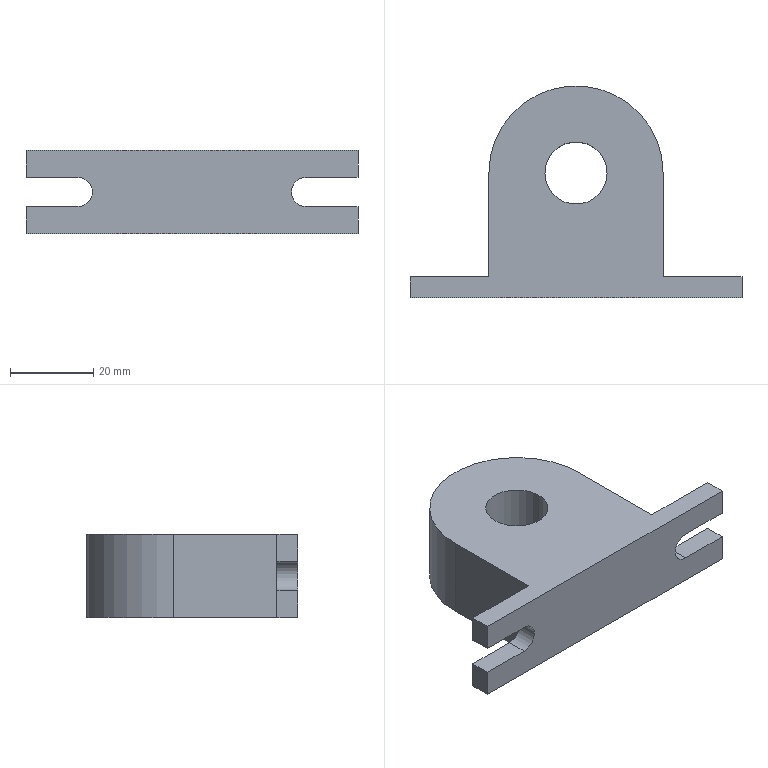Part | SolidWorks | features Extrusion 1, ICE 1 | 1 solid | 21 faces | box 80 x 51 x 20 mm | volume 38253 mm3 | plane 15 | cylinder 6 | commonest cylinder face diameters 7 x3 15 x2 42 x1
STEP:
#1=CARTESIAN_POINT('',(24.,-30.,10.));
#2=VERTEX_POINT('',#1);
#3=CARTESIAN_POINT('',(27.5,-30.,13.5));
#4=VERTEX_POINT('',#3);
#5=CARTESIAN_POINT('',(27.5,-30.,10.));
#6=DIRECTION('',(0.,1.,0.));
#7=DIRECTION('',(1.,0.,0.));
#8=AXIS2_PLACEMENT_3D('',#5,#6,#7);
#9=CIRCLE('',#8,3.5);
#10=EDGE_CURVE('',#2,#4,#9,.T.);
#11=ORIENTED_EDGE('',*,*,#10,.F.);
#12=CARTESIAN_POINT('',(24.,-25.,10.));
#13=VERTEX_POINT('',#12);
#14=CARTESIAN_POINT('',(24.,-30.,10.));
#15=DIRECTION('',(0.,1.,0.));
#16=VECTOR('',#15,1000.);
#17=LINE('',#14,#16);
#18=EDGE_CURVE('',#2,#13,#17,.T.);
#19=ORIENTED_EDGE('',*,*,#18,.T.);
#20=CARTESIAN_POINT('',(27.5,-25.,13.5));
#21=VERTEX_POINT('',#20);
#22=CARTESIAN_POINT('',(27.5,-25.,10.));
#23=DIRECTION('',(0.,1.,0.));
#24=DIRECTION('',(1.,0.,0.));
#25=AXIS2_PLACEMENT_3D('',#22,#23,#24);
#26=CIRCLE('',#25,3.5);
#27=EDGE_CURVE('',#13,#21,#26,.T.);
#28=ORIENTED_EDGE('',*,*,#27,.T.);
#29=CARTESIAN_POINT('',(27.5,-30.,13.5));
#30=DIRECTION('',(0.,1.,0.));
#31=VECTOR('',#30,1000.);
#32=LINE('',#29,#31);
#33=EDGE_CURVE('',#4,#21,#32,.T.);
#34=ORIENTED_EDGE('',*,*,#33,.F.);
#35=EDGE_LOOP('',(#11,#19,#28,#34));
#36=FACE_OUTER_BOUND('',#35,.T.);
#37=CARTESIAN_POINT('',(27.5,-30.,10.));
#38=DIRECTION('',(0.,1.,0.));
#39=DIRECTION('',(-1.,0.,0.));
#40=AXIS2_PLACEMENT_3D('',#37,#38,#39);
#41=CYLINDRICAL_SURFACE('',#40,3.5);
#42=ADVANCED_FACE('',(#36),#41,.F.);
#43=CARTESIAN_POINT('',(-7.5,0.,20.));
#44=VERTEX_POINT('',#43);
#45=CARTESIAN_POINT('',(7.5,0.,20.));
#46=VERTEX_POINT('',#45);
#47=CARTESIAN_POINT('',(0.,0.,20.));
#48=DIRECTION('',(0.,0.,1.));
#49=DIRECTION('',(1.,0.,0.));
#50=AXIS2_PLACEMENT_3D('',#47,#48,#49);
#51=CIRCLE('',#50,7.5);
#52=EDGE_CURVE('',#44,#46,#51,.T.);
#53=ORIENTED_EDGE('',*,*,#52,.T.);
#54=CARTESIAN_POINT('',(7.5,0.,0.));
#55=VERTEX_POINT('',#54);
#56=CARTESIAN_POINT('',(7.5,0.,20.));
#57=DIRECTION('',(0.,0.,-1.));
#58=VECTOR('',#57,1000.);
#59=LINE('',#56,#58);
#60=EDGE_CURVE('',#46,#55,#59,.T.);
#61=ORIENTED_EDGE('',*,*,#60,.T.);
#62=CARTESIAN_POINT('',(-7.5,0.,0.));
#63=VERTEX_POINT('',#62);
#64=CARTESIAN_POINT('',(0.,0.,0.));
#65=DIRECTION('',(0.,0.,1.));
#66=DIRECTION('',(1.,0.,0.));
#67=AXIS2_PLACEMENT_3D('',#64,#65,#66);
#68=CIRCLE('',#67,7.5);
#69=EDGE_CURVE('',#63,#55,#68,.T.);
#70=ORIENTED_EDGE('',*,*,#69,.F.);
#71=CARTESIAN_POINT('',(-7.5,0.,20.));
#72=DIRECTION('',(0.,0.,-1.));
#73=VECTOR('',#72,1000.);
#74=LINE('',#71,#73);
#75=EDGE_CURVE('',#44,#63,#74,.T.);
#76=ORIENTED_EDGE('',*,*,#75,.F.);
#77=EDGE_LOOP('',(#53,#61,#70,#76));
#78=FACE_OUTER_BOUND('',#77,.T.);
#79=CARTESIAN_POINT('',(0.,0.,20.));
#80=DIRECTION('',(0.,0.,-1.));
#81=DIRECTION('',(-1.,0.,0.));
#82=AXIS2_PLACEMENT_3D('',#79,#80,#81);
#83=CYLINDRICAL_SURFACE('',#82,7.5);
#84=ADVANCED_FACE('',(#78),#83,.F.);
#85=CARTESIAN_POINT('',(40.,-25.,6.5));
#86=VERTEX_POINT('',#85);
#87=CARTESIAN_POINT('',(40.,-25.,0.));
#88=VERTEX_POINT('',#87);
#89=CARTESIAN_POINT('',(40.,-25.,20.));
#90=DIRECTION('',(0.,0.,-1.));
#91=VECTOR('',#90,1000.);
#92=LINE('',#89,#91);
#93=EDGE_CURVE('',#86,#88,#92,.T.);
#94=ORIENTED_EDGE('',*,*,#93,.F.);
#95=CARTESIAN_POINT('',(40.,-30.,6.5));
#96=VERTEX_POINT('',#95);
#97=CARTESIAN_POINT('',(40.,-30.,6.5));
#98=DIRECTION('',(0.,1.,0.));
#99=VECTOR('',#98,1000.);
#100=LINE('',#97,#99);
#101=EDGE_CURVE('',#96,#86,#100,.T.);
#102=ORIENTED_EDGE('',*,*,#101,.F.);
#103=CARTESIAN_POINT('',(40.,-30.,0.));
#104=VERTEX_POINT('',#103);
#105=CARTESIAN_POINT('',(40.,-30.,20.));
#106=DIRECTION('',(0.,0.,-1.));
#107=VECTOR('',#106,1000.);
#108=LINE('',#105,#107);
#109=EDGE_CURVE('',#96,#104,#108,.T.);
#110=ORIENTED_EDGE('',*,*,#109,.T.);
#111=CARTESIAN_POINT('',(40.,-30.,0.));
#112=DIRECTION('',(0.,1.,0.));
#113=VECTOR('',#112,1000.);
#114=LINE('',#111,#113);
#115=EDGE_CURVE('',#104,#88,#114,.T.);
#116=ORIENTED_EDGE('',*,*,#115,.T.);
#117=EDGE_LOOP('',(#94,#102,#110,#116));
#118=FACE_OUTER_BOUND('',#117,.T.);
#119=CARTESIAN_POINT('',(40.,-30.,20.));
#120=DIRECTION('',(-1.,0.,0.));
#121=DIRECTION('',(0.,0.,1.));
#122=AXIS2_PLACEMENT_3D('',#119,#120,#121);
#123=PLANE('',#122);
#124=ADVANCED_FACE('',(#118),#123,.F.);
#125=CARTESIAN_POINT('',(-40.,-25.,20.));
#126=VERTEX_POINT('',#125);
#127=CARTESIAN_POINT('',(-40.,-25.,13.5));
#128=VERTEX_POINT('',#127);
#129=CARTESIAN_POINT('',(-40.,-25.,20.));
#130=DIRECTION('',(0.,0.,-1.));
#131=VECTOR('',#130,1000.);
#132=LINE('',#129,#131);
#133=EDGE_CURVE('',#126,#128,#132,.T.);
#134=ORIENTED_EDGE('',*,*,#133,.T.);
#135=CARTESIAN_POINT('',(-40.,-30.,13.5));
#136=VERTEX_POINT('',#135);
#137=CARTESIAN_POINT('',(-40.,-30.,13.5));
#138=DIRECTION('',(0.,1.,0.));
#139=VECTOR('',#138,1000.);
#140=LINE('',#137,#139);
#141=EDGE_CURVE('',#136,#128,#140,.T.);
#142=ORIENTED_EDGE('',*,*,#141,.F.);
#143=CARTESIAN_POINT('',(-40.,-30.,20.));
#144=VERTEX_POINT('',#143);
#145=CARTESIAN_POINT('',(-40.,-30.,20.));
#146=DIRECTION('',(0.,0.,-1.));
#147=VECTOR('',#146,1000.);
#148=LINE('',#145,#147);
#149=EDGE_CURVE('',#144,#136,#148,.T.);
#150=ORIENTED_EDGE('',*,*,#149,.F.);
#151=CARTESIAN_POINT('',(-40.,-30.,20.));
#152=DIRECTION('',(0.,-1.,0.));
#153=VECTOR('',#152,1000.);
#154=LINE('',#151,#153);
#155=EDGE_CURVE('',#126,#144,#154,.T.);
#156=ORIENTED_EDGE('',*,*,#155,.F.);
#157=EDGE_LOOP('',(#134,#142,#150,#156));
#158=FACE_OUTER_BOUND('',#157,.T.);
#159=CARTESIAN_POINT('',(-40.,-30.,20.));
#160=DIRECTION('',(1.,0.,0.));
#161=DIRECTION('',(0.,0.,-1.));
#162=AXIS2_PLACEMENT_3D('',#159,#160,#161);
#163=PLANE('',#162);
#164=ADVANCED_FACE('',(#158),#163,.F.);
#165=CARTESIAN_POINT('',(21.,0.,20.));
#166=VERTEX_POINT('',#165);
#167=CARTESIAN_POINT('',(-21.,0.,20.));
#168=VERTEX_POINT('',#167);
#169=CARTESIAN_POINT('',(0.,0.,20.));
#170=DIRECTION('',(0.,0.,1.));
#171=DIRECTION('',(1.,0.,0.));
#172=AXIS2_PLACEMENT_3D('',#169,#170,#171);
#173=CIRCLE('',#172,21.);
#174=EDGE_CURVE('',#166,#168,#173,.T.);
#175=ORIENTED_EDGE('',*,*,#174,.T.);
#176=CARTESIAN_POINT('',(-21.,-25.,20.));
#177=VERTEX_POINT('',#176);
#178=CARTESIAN_POINT('',(-21.,0.,20.));
#179=DIRECTION('',(0.,-1.,0.));
#180=VECTOR('',#179,1000.);
#181=LINE('',#178,#180);
#182=EDGE_CURVE('',#168,#177,#181,.T.);
#183=ORIENTED_EDGE('',*,*,#182,.T.);
#184=CARTESIAN_POINT('',(-40.,-25.,20.));
#185=DIRECTION('',(-1.,0.,0.));
#186=VECTOR('',#185,1000.);
#187=LINE('',#184,#186);
#188=EDGE_CURVE('',#177,#126,#187,.T.);
#189=ORIENTED_EDGE('',*,*,#188,.T.);
#190=ORIENTED_EDGE('',*,*,#155,.T.);
#191=CARTESIAN_POINT('',(40.,-30.,20.));
#192=VERTEX_POINT('',#191);
#193=CARTESIAN_POINT('',(-21.,-30.,20.));
#194=DIRECTION('',(1.,0.,0.));
#195=VECTOR('',#194,1000.);
#196=LINE('',#193,#195);
#197=EDGE_CURVE('',#144,#192,#196,.T.);
#198=ORIENTED_EDGE('',*,*,#197,.T.);
#199=CARTESIAN_POINT('',(40.,-25.,20.));
#200=VERTEX_POINT('',#199);
#201=CARTESIAN_POINT('',(40.,-30.,20.));
#202=DIRECTION('',(0.,1.,0.));
#203=VECTOR('',#202,1000.);
#204=LINE('',#201,#203);
#205=EDGE_CURVE('',#192,#200,#204,.T.);
#206=ORIENTED_EDGE('',*,*,#205,.T.);
#207=CARTESIAN_POINT('',(21.,-25.,20.));
#208=VERTEX_POINT('',#207);
#209=CARTESIAN_POINT('',(40.,-25.,20.));
#210=DIRECTION('',(-1.,0.,0.));
#211=VECTOR('',#210,1000.);
#212=LINE('',#209,#211);
#213=EDGE_CURVE('',#200,#208,#212,.T.);
#214=ORIENTED_EDGE('',*,*,#213,.T.);
#215=CARTESIAN_POINT('',(21.,0.,20.));
#216=DIRECTION('',(0.,1.,0.));
#217=VECTOR('',#216,1000.);
#218=LINE('',#215,#217);
#219=EDGE_CURVE('',#208,#166,#218,.T.);
#220=ORIENTED_EDGE('',*,*,#219,.T.);
#221=EDGE_LOOP('',(#175,#183,#189,#190,#198,#206,#214,#220));
#222=FACE_OUTER_BOUND('',#221,.T.);
#223=ORIENTED_EDGE('',*,*,#52,.F.);
#224=CARTESIAN_POINT('',(0.,0.,20.));
#225=DIRECTION('',(0.,0.,1.));
#226=DIRECTION('',(1.,0.,0.));
#227=AXIS2_PLACEMENT_3D('',#224,#225,#226);
#228=CIRCLE('',#227,7.5);
#229=EDGE_CURVE('',#46,#44,#228,.T.);
#230=ORIENTED_EDGE('',*,*,#229,.F.);
#231=EDGE_LOOP('',(#223,#230));
#232=FACE_BOUND('',#231,.T.);
#233=CARTESIAN_POINT('',(0.,0.,20.));
#234=DIRECTION('',(0.,0.,1.));
#235=DIRECTION('',(1.,0.,0.));
#236=AXIS2_PLACEMENT_3D('',#233,#234,#235);
#237=PLANE('',#236);
#238=ADVANCED_FACE('',(#222,#232),#237,.T.);
#239=CARTESIAN_POINT('',(21.,0.,0.));
#240=VERTEX_POINT('',#239);
#241=CARTESIAN_POINT('',(-21.,0.,0.));
#242=VERTEX_POINT('',#241);
#243=CARTESIAN_POINT('',(0.,0.,0.));
#244=DIRECTION('',(0.,0.,1.));
#245=DIRECTION('',(1.,0.,0.));
#246=AXIS2_PLACEMENT_3D('',#243,#244,#245);
#247=CIRCLE('',#246,21.);
#248=EDGE_CURVE('',#240,#242,#247,.T.);
#249=ORIENTED_EDGE('',*,*,#248,.F.);
#250=CARTESIAN_POINT('',(21.,-25.,0.));
#251=VERTEX_POINT('',#250);
#252=CARTESIAN_POINT('',(21.,0.,0.));
#253=DIRECTION('',(0.,1.,0.));
#254=VECTOR('',#253,1000.);
#255=LINE('',#252,#254);
#256=EDGE_CURVE('',#251,#240,#255,.T.);
#257=ORIENTED_EDGE('',*,*,#256,.F.);
#258=CARTESIAN_POINT('',(40.,-25.,0.));
#259=DIRECTION('',(-1.,0.,0.));
#260=VECTOR('',#259,1000.);
#261=LINE('',#258,#260);
#262=EDGE_CURVE('',#88,#251,#261,.T.);
#263=ORIENTED_EDGE('',*,*,#262,.F.);
#264=ORIENTED_EDGE('',*,*,#115,.F.);
#265=CARTESIAN_POINT('',(-40.,-30.,0.));
#266=VERTEX_POINT('',#265);
#267=CARTESIAN_POINT('',(21.,-30.,0.));
#268=DIRECTION('',(1.,0.,0.));
#269=VECTOR('',#268,1000.);
#270=LINE('',#267,#269);
#271=EDGE_CURVE('',#266,#104,#270,.T.);
#272=ORIENTED_EDGE('',*,*,#271,.F.);
#273=CARTESIAN_POINT('',(-40.,-25.,0.));
#274=VERTEX_POINT('',#273);
#275=CARTESIAN_POINT('',(-40.,-30.,0.));
#276=DIRECTION('',(0.,-1.,0.));
#277=VECTOR('',#276,1000.);
#278=LINE('',#275,#277);
#279=EDGE_CURVE('',#274,#266,#278,.T.);
#280=ORIENTED_EDGE('',*,*,#279,.F.);
#281=CARTESIAN_POINT('',(-21.,-25.,0.));
#282=VERTEX_POINT('',#281);
#283=CARTESIAN_POINT('',(-40.,-25.,0.));
#284=DIRECTION('',(-1.,0.,0.));
#285=VECTOR('',#284,1000.);
#286=LINE('',#283,#285);
#287=EDGE_CURVE('',#282,#274,#286,.T.);
#288=ORIENTED_EDGE('',*,*,#287,.F.);
#289=CARTESIAN_POINT('',(-21.,0.,0.));
#290=DIRECTION('',(0.,-1.,0.));
#291=VECTOR('',#290,1000.);
#292=LINE('',#289,#291);
#293=EDGE_CURVE('',#242,#282,#292,.T.);
#294=ORIENTED_EDGE('',*,*,#293,.F.);
#295=EDGE_LOOP('',(#249,#257,#263,#264,#272,#280,#288,#294));
#296=FACE_OUTER_BOUND('',#295,.T.);
#297=ORIENTED_EDGE('',*,*,#69,.T.);
#298=CARTESIAN_POINT('',(0.,0.,0.));
#299=DIRECTION('',(0.,0.,1.));
#300=DIRECTION('',(1.,0.,0.));
#301=AXIS2_PLACEMENT_3D('',#298,#299,#300);
#302=CIRCLE('',#301,7.5);
#303=EDGE_CURVE('',#55,#63,#302,.T.);
#304=ORIENTED_EDGE('',*,*,#303,.T.);
#305=EDGE_LOOP('',(#297,#304));
#306=FACE_BOUND('',#305,.T.);
#307=CARTESIAN_POINT('',(0.,0.,0.));
#308=DIRECTION('',(0.,0.,1.));
#309=DIRECTION('',(1.,0.,0.));
#310=AXIS2_PLACEMENT_3D('',#307,#308,#309);
#311=PLANE('',#310);
#312=ADVANCED_FACE('',(#296,#306),#311,.F.);
#313=ORIENTED_EDGE('',*,*,#248,.T.);
#314=CARTESIAN_POINT('',(-21.,0.,20.));
#315=DIRECTION('',(0.,0.,-1.));
#316=VECTOR('',#315,1000.);
#317=LINE('',#314,#316);
#318=EDGE_CURVE('',#168,#242,#317,.T.);
#319=ORIENTED_EDGE('',*,*,#318,.F.);
#320=ORIENTED_EDGE('',*,*,#174,.F.);
#321=CARTESIAN_POINT('',(21.,0.,20.));
#322=DIRECTION('',(0.,0.,-1.));
#323=VECTOR('',#322,1000.);
#324=LINE('',#321,#323);
#325=EDGE_CURVE('',#166,#240,#324,.T.);
#326=ORIENTED_EDGE('',*,*,#325,.T.);
#327=EDGE_LOOP('',(#313,#319,#320,#326));
#328=FACE_OUTER_BOUND('',#327,.T.);
#329=CARTESIAN_POINT('',(0.,0.,20.));
#330=DIRECTION('',(0.,0.,-1.));
#331=DIRECTION('',(-1.,0.,0.));
#332=AXIS2_PLACEMENT_3D('',#329,#330,#331);
#333=CYLINDRICAL_SURFACE('',#332,21.);
#334=ADVANCED_FACE('',(#328),#333,.T.);
#335=ORIENTED_EDGE('',*,*,#293,.T.);
#336=CARTESIAN_POINT('',(-21.,-25.,20.));
#337=DIRECTION('',(0.,0.,-1.));
#338=VECTOR('',#337,1000.);
#339=LINE('',#336,#338);
#340=EDGE_CURVE('',#177,#282,#339,.T.);
#341=ORIENTED_EDGE('',*,*,#340,.F.);
#342=ORIENTED_EDGE('',*,*,#182,.F.);
#343=ORIENTED_EDGE('',*,*,#318,.T.);
#344=EDGE_LOOP('',(#335,#341,#342,#343));
#345=FACE_OUTER_BOUND('',#344,.T.);
#346=CARTESIAN_POINT('',(-21.,0.,20.));
#347=DIRECTION('',(1.,0.,0.));
#348=DIRECTION('',(0.,1.,0.));
#349=AXIS2_PLACEMENT_3D('',#346,#347,#348);
#350=PLANE('',#349);
#351=ADVANCED_FACE('',(#345),#350,.F.);
#352=CARTESIAN_POINT('',(-27.5,-25.,13.5));
#353=VERTEX_POINT('',#352);
#354=CARTESIAN_POINT('',(-27.5,-25.,6.5));
#355=VERTEX_POINT('',#354);
#356=CARTESIAN_POINT('',(-27.5,-25.,10.));
#357=DIRECTION('',(0.,1.,0.));
#358=DIRECTION('',(-1.,0.,0.));
#359=AXIS2_PLACEMENT_3D('',#356,#357,#358);
#360=CIRCLE('',#359,3.5);
#361=EDGE_CURVE('',#353,#355,#360,.T.);
#362=ORIENTED_EDGE('',*,*,#361,.F.);
#363=CARTESIAN_POINT('',(-40.,-25.,13.5));
#364=DIRECTION('',(1.,0.,0.));
#365=VECTOR('',#364,1000.);
#366=LINE('',#363,#365);
#367=EDGE_CURVE('',#128,#353,#366,.T.);
#368=ORIENTED_EDGE('',*,*,#367,.F.);
#369=ORIENTED_EDGE('',*,*,#133,.F.);
#370=ORIENTED_EDGE('',*,*,#188,.F.);
#371=ORIENTED_EDGE('',*,*,#340,.T.);
#372=ORIENTED_EDGE('',*,*,#287,.T.);
#373=CARTESIAN_POINT('',(-40.,-25.,6.5));
#374=VERTEX_POINT('',#373);
#375=CARTESIAN_POINT('',(-40.,-25.,20.));
#376=DIRECTION('',(0.,0.,-1.));
#377=VECTOR('',#376,1000.);
#378=LINE('',#375,#377);
#379=EDGE_CURVE('',#374,#274,#378,.T.);
#380=ORIENTED_EDGE('',*,*,#379,.F.);
#381=CARTESIAN_POINT('',(-27.5,-25.,6.5));
#382=DIRECTION('',(-1.,0.,0.));
#383=VECTOR('',#382,1000.);
#384=LINE('',#381,#383);
#385=EDGE_CURVE('',#355,#374,#384,.T.);
#386=ORIENTED_EDGE('',*,*,#385,.F.);
#387=EDGE_LOOP('',(#362,#368,#369,#370,#371,#372,#380,#386));
#388=FACE_OUTER_BOUND('',#387,.T.);
#389=CARTESIAN_POINT('',(-40.,-25.,20.));
#390=DIRECTION('',(0.,-1.,0.));
#391=DIRECTION('',(1.,0.,0.));
#392=AXIS2_PLACEMENT_3D('',#389,#390,#391);
#393=PLANE('',#392);
#394=ADVANCED_FACE('',(#388),#393,.F.);
#395=CARTESIAN_POINT('',(-40.,-30.,6.5));
#396=VERTEX_POINT('',#395);
#397=CARTESIAN_POINT('',(-40.,-30.,20.));
#398=DIRECTION('',(0.,0.,-1.));
#399=VECTOR('',#398,1000.);
#400=LINE('',#397,#399);
#401=EDGE_CURVE('',#396,#266,#400,.T.);
#402=ORIENTED_EDGE('',*,*,#401,.F.);
#403=CARTESIAN_POINT('',(-40.,-30.,6.5));
#404=DIRECTION('',(0.,1.,0.));
#405=VECTOR('',#404,1000.);
#406=LINE('',#403,#405);
#407=EDGE_CURVE('',#396,#374,#406,.T.);
#408=ORIENTED_EDGE('',*,*,#407,.T.);
#409=ORIENTED_EDGE('',*,*,#379,.T.);
#410=ORIENTED_EDGE('',*,*,#279,.T.);
#411=EDGE_LOOP('',(#402,#408,#409,#410));
#412=FACE_OUTER_BOUND('',#411,.T.);
#413=CARTESIAN_POINT('',(-40.,-30.,20.));
#414=DIRECTION('',(1.,0.,0.));
#415=DIRECTION('',(0.,0.,-1.));
#416=AXIS2_PLACEMENT_3D('',#413,#414,#415);
#417=PLANE('',#416);
#418=ADVANCED_FACE('',(#412),#417,.F.);
#419=ORIENTED_EDGE('',*,*,#109,.F.);
#420=CARTESIAN_POINT('',(27.5,-30.,6.5));
#421=VERTEX_POINT('',#420);
#422=CARTESIAN_POINT('',(27.5,-30.,6.5));
#423=DIRECTION('',(-1.,0.,0.));
#424=VECTOR('',#423,1000.);
#425=LINE('',#422,#424);
#426=EDGE_CURVE('',#96,#421,#425,.T.);
#427=ORIENTED_EDGE('',*,*,#426,.T.);
#428=CARTESIAN_POINT('',(27.5,-30.,10.));
#429=DIRECTION('',(0.,1.,0.));
#430=DIRECTION('',(1.,0.,0.));
#431=AXIS2_PLACEMENT_3D('',#428,#429,#430);
#432=CIRCLE('',#431,3.5);
#433=EDGE_CURVE('',#421,#2,#432,.T.);
#434=ORIENTED_EDGE('',*,*,#433,.T.);
#435=ORIENTED_EDGE('',*,*,#10,.T.);
#436=CARTESIAN_POINT('',(40.,-30.,13.5));
#437=VERTEX_POINT('',#436);
#438=CARTESIAN_POINT('',(40.,-30.,13.5));
#439=DIRECTION('',(1.,0.,0.));
#440=VECTOR('',#439,1000.);
#441=LINE('',#438,#440);
#442=EDGE_CURVE('',#4,#437,#441,.T.);
#443=ORIENTED_EDGE('',*,*,#442,.T.);
#444=CARTESIAN_POINT('',(40.,-30.,20.));
#445=DIRECTION('',(0.,0.,-1.));
#446=VECTOR('',#445,1000.);
#447=LINE('',#444,#446);
#448=EDGE_CURVE('',#192,#437,#447,.T.);
#449=ORIENTED_EDGE('',*,*,#448,.F.);
#450=ORIENTED_EDGE('',*,*,#197,.F.);
#451=ORIENTED_EDGE('',*,*,#149,.T.);
#452=CARTESIAN_POINT('',(-27.5,-30.,13.5));
#453=VERTEX_POINT('',#452);
#454=CARTESIAN_POINT('',(-40.,-30.,13.5));
#455=DIRECTION('',(1.,0.,0.));
#456=VECTOR('',#455,1000.);
#457=LINE('',#454,#456);
#458=EDGE_CURVE('',#136,#453,#457,.T.);
#459=ORIENTED_EDGE('',*,*,#458,.T.);
#460=CARTESIAN_POINT('',(-27.5,-30.,6.5));
#461=VERTEX_POINT('',#460);
#462=CARTESIAN_POINT('',(-27.5,-30.,10.));
#463=DIRECTION('',(0.,1.,0.));
#464=DIRECTION('',(-1.,0.,0.));
#465=AXIS2_PLACEMENT_3D('',#462,#463,#464);
#466=CIRCLE('',#465,3.5);
#467=EDGE_CURVE('',#453,#461,#466,.T.);
#468=ORIENTED_EDGE('',*,*,#467,.T.);
#469=CARTESIAN_POINT('',(-27.5,-30.,6.5));
#470=DIRECTION('',(-1.,0.,0.));
#471=VECTOR('',#470,1000.);
#472=LINE('',#469,#471);
#473=EDGE_CURVE('',#461,#396,#472,.T.);
#474=ORIENTED_EDGE('',*,*,#473,.T.);
#475=ORIENTED_EDGE('',*,*,#401,.T.);
#476=ORIENTED_EDGE('',*,*,#271,.T.);
#477=EDGE_LOOP('',(#419,#427,#434,#435,#443,#449,#450,#451,#459,#468,#474,#475,#476));
#478=FACE_OUTER_BOUND('',#477,.T.);
#479=CARTESIAN_POINT('',(21.,-30.,20.));
#480=DIRECTION('',(0.,1.,0.));
#481=DIRECTION('',(-1.,0.,0.));
#482=AXIS2_PLACEMENT_3D('',#479,#480,#481);
#483=PLANE('',#482);
#484=ADVANCED_FACE('',(#478),#483,.F.);
#485=ORIENTED_EDGE('',*,*,#448,.T.);
#486=CARTESIAN_POINT('',(40.,-25.,13.5));
#487=VERTEX_POINT('',#486);
#488=CARTESIAN_POINT('',(40.,-30.,13.5));
#489=DIRECTION('',(0.,1.,0.));
#490=VECTOR('',#489,1000.);
#491=LINE('',#488,#490);
#492=EDGE_CURVE('',#437,#487,#491,.T.);
#493=ORIENTED_EDGE('',*,*,#492,.T.);
#494=CARTESIAN_POINT('',(40.,-25.,20.));
#495=DIRECTION('',(0.,0.,-1.));
#496=VECTOR('',#495,1000.);
#497=LINE('',#494,#496);
#498=EDGE_CURVE('',#200,#487,#497,.T.);
#499=ORIENTED_EDGE('',*,*,#498,.F.);
#500=ORIENTED_EDGE('',*,*,#205,.F.);
#501=EDGE_LOOP('',(#485,#493,#499,#500));
#502=FACE_OUTER_BOUND('',#501,.T.);
#503=CARTESIAN_POINT('',(40.,-30.,20.));
#504=DIRECTION('',(-1.,0.,0.));
#505=DIRECTION('',(0.,0.,1.));
#506=AXIS2_PLACEMENT_3D('',#503,#504,#505);
#507=PLANE('',#506);
#508=ADVANCED_FACE('',(#502),#507,.F.);
#509=CARTESIAN_POINT('',(27.5,-25.,6.5));
#510=VERTEX_POINT('',#509);
#511=CARTESIAN_POINT('',(27.5,-25.,10.));
#512=DIRECTION('',(0.,1.,0.));
#513=DIRECTION('',(1.,0.,0.));
#514=AXIS2_PLACEMENT_3D('',#511,#512,#513);
#515=CIRCLE('',#514,3.5);
#516=EDGE_CURVE('',#510,#13,#515,.T.);
#517=ORIENTED_EDGE('',*,*,#516,.F.);
#518=CARTESIAN_POINT('',(27.5,-25.,6.5));
#519=DIRECTION('',(-1.,0.,0.));
#520=VECTOR('',#519,1000.);
#521=LINE('',#518,#520);
#522=EDGE_CURVE('',#86,#510,#521,.T.);
#523=ORIENTED_EDGE('',*,*,#522,.F.);
#524=ORIENTED_EDGE('',*,*,#93,.T.);
#525=ORIENTED_EDGE('',*,*,#262,.T.);
#526=CARTESIAN_POINT('',(21.,-25.,20.));
#527=DIRECTION('',(0.,0.,-1.));
#528=VECTOR('',#527,1000.);
#529=LINE('',#526,#528);
#530=EDGE_CURVE('',#208,#251,#529,.T.);
#531=ORIENTED_EDGE('',*,*,#530,.F.);
#532=ORIENTED_EDGE('',*,*,#213,.F.);
#533=ORIENTED_EDGE('',*,*,#498,.T.);
#534=CARTESIAN_POINT('',(40.,-25.,13.5));
#535=DIRECTION('',(1.,0.,0.));
#536=VECTOR('',#535,1000.);
#537=LINE('',#534,#536);
#538=EDGE_CURVE('',#21,#487,#537,.T.);
#539=ORIENTED_EDGE('',*,*,#538,.F.);
#540=ORIENTED_EDGE('',*,*,#27,.F.);
#541=EDGE_LOOP('',(#517,#523,#524,#525,#531,#532,#533,#539,#540));
#542=FACE_OUTER_BOUND('',#541,.T.);
#543=CARTESIAN_POINT('',(40.,-25.,20.));
#544=DIRECTION('',(0.,-1.,0.));
#545=DIRECTION('',(1.,0.,0.));
#546=AXIS2_PLACEMENT_3D('',#543,#544,#545);
#547=PLANE('',#546);
#548=ADVANCED_FACE('',(#542),#547,.F.);
#549=ORIENTED_EDGE('',*,*,#256,.T.);
#550=ORIENTED_EDGE('',*,*,#325,.F.);
#551=ORIENTED_EDGE('',*,*,#219,.F.);
#552=ORIENTED_EDGE('',*,*,#530,.T.);
#553=EDGE_LOOP('',(#549,#550,#551,#552));
#554=FACE_OUTER_BOUND('',#553,.T.);
#555=CARTESIAN_POINT('',(21.,0.,20.));
#556=DIRECTION('',(-1.,0.,0.));
#557=DIRECTION('',(0.,-1.,0.));
#558=AXIS2_PLACEMENT_3D('',#555,#556,#557);
#559=PLANE('',#558);
#560=ADVANCED_FACE('',(#554),#559,.F.);
#561=ORIENTED_EDGE('',*,*,#60,.F.);
#562=ORIENTED_EDGE('',*,*,#229,.T.);
#563=ORIENTED_EDGE('',*,*,#75,.T.);
#564=ORIENTED_EDGE('',*,*,#303,.F.);
#565=EDGE_LOOP('',(#561,#562,#563,#564));
#566=FACE_OUTER_BOUND('',#565,.T.);
#567=CARTESIAN_POINT('',(0.,0.,20.));
#568=DIRECTION('',(0.,0.,-1.));
#569=DIRECTION('',(-1.,0.,0.));
#570=AXIS2_PLACEMENT_3D('',#567,#568,#569);
#571=CYLINDRICAL_SURFACE('',#570,7.5);
#572=ADVANCED_FACE('',(#566),#571,.F.);
#573=ORIENTED_EDGE('',*,*,#361,.T.);
#574=CARTESIAN_POINT('',(-27.5,-30.,6.5));
#575=DIRECTION('',(0.,1.,0.));
#576=VECTOR('',#575,1000.);
#577=LINE('',#574,#576);
#578=EDGE_CURVE('',#461,#355,#577,.T.);
#579=ORIENTED_EDGE('',*,*,#578,.F.);
#580=ORIENTED_EDGE('',*,*,#467,.F.);
#581=CARTESIAN_POINT('',(-27.5,-30.,13.5));
#582=DIRECTION('',(0.,1.,0.));
#583=VECTOR('',#582,1000.);
#584=LINE('',#581,#583);
#585=EDGE_CURVE('',#453,#353,#584,.T.);
#586=ORIENTED_EDGE('',*,*,#585,.T.);
#587=EDGE_LOOP('',(#573,#579,#580,#586));
#588=FACE_OUTER_BOUND('',#587,.T.);
#589=CARTESIAN_POINT('',(-27.5,-30.,10.));
#590=DIRECTION('',(0.,1.,0.));
#591=DIRECTION('',(-1.,0.,0.));
#592=AXIS2_PLACEMENT_3D('',#589,#590,#591);
#593=CYLINDRICAL_SURFACE('',#592,3.5);
#594=ADVANCED_FACE('',(#588),#593,.F.);
#595=ORIENTED_EDGE('',*,*,#367,.T.);
#596=ORIENTED_EDGE('',*,*,#585,.F.);
#597=ORIENTED_EDGE('',*,*,#458,.F.);
#598=ORIENTED_EDGE('',*,*,#141,.T.);
#599=EDGE_LOOP('',(#595,#596,#597,#598));
#600=FACE_OUTER_BOUND('',#599,.T.);
#601=CARTESIAN_POINT('',(-40.,-30.,13.5));
#602=DIRECTION('',(0.,0.,1.));
#603=DIRECTION('',(1.,0.,0.));
#604=AXIS2_PLACEMENT_3D('',#601,#602,#603);
#605=PLANE('',#604);
#606=ADVANCED_FACE('',(#600),#605,.F.);
#607=ORIENTED_EDGE('',*,*,#385,.T.);
#608=ORIENTED_EDGE('',*,*,#407,.F.);
#609=ORIENTED_EDGE('',*,*,#473,.F.);
#610=ORIENTED_EDGE('',*,*,#578,.T.);
#611=EDGE_LOOP('',(#607,#608,#609,#610));
#612=FACE_OUTER_BOUND('',#611,.T.);
#613=CARTESIAN_POINT('',(-27.5,-30.,6.5));
#614=DIRECTION('',(0.,0.,-1.));
#615=DIRECTION('',(-1.,0.,0.));
#616=AXIS2_PLACEMENT_3D('',#613,#614,#615);
#617=PLANE('',#616);
#618=ADVANCED_FACE('',(#612),#617,.F.);
#619=ORIENTED_EDGE('',*,*,#18,.F.);
#620=ORIENTED_EDGE('',*,*,#433,.F.);
#621=CARTESIAN_POINT('',(27.5,-30.,6.5));
#622=DIRECTION('',(0.,1.,0.));
#623=VECTOR('',#622,1000.);
#624=LINE('',#621,#623);
#625=EDGE_CURVE('',#421,#510,#624,.T.);
#626=ORIENTED_EDGE('',*,*,#625,.T.);
#627=ORIENTED_EDGE('',*,*,#516,.T.);
#628=EDGE_LOOP('',(#619,#620,#626,#627));
#629=FACE_OUTER_BOUND('',#628,.T.);
#630=CARTESIAN_POINT('',(27.5,-30.,10.));
#631=DIRECTION('',(0.,1.,0.));
#632=DIRECTION('',(-1.,0.,0.));
#633=AXIS2_PLACEMENT_3D('',#630,#631,#632);
#634=CYLINDRICAL_SURFACE('',#633,3.5);
#635=ADVANCED_FACE('',(#629),#634,.F.);
#636=ORIENTED_EDGE('',*,*,#522,.T.);
#637=ORIENTED_EDGE('',*,*,#625,.F.);
#638=ORIENTED_EDGE('',*,*,#426,.F.);
#639=ORIENTED_EDGE('',*,*,#101,.T.);
#640=EDGE_LOOP('',(#636,#637,#638,#639));
#641=FACE_OUTER_BOUND('',#640,.T.);
#642=CARTESIAN_POINT('',(27.5,-30.,6.5));
#643=DIRECTION('',(0.,0.,-1.));
#644=DIRECTION('',(-1.,0.,0.));
#645=AXIS2_PLACEMENT_3D('',#642,#643,#644);
#646=PLANE('',#645);
#647=ADVANCED_FACE('',(#641),#646,.F.);
#648=ORIENTED_EDGE('',*,*,#538,.T.);
#649=ORIENTED_EDGE('',*,*,#492,.F.);
#650=ORIENTED_EDGE('',*,*,#442,.F.);
#651=ORIENTED_EDGE('',*,*,#33,.T.);
#652=EDGE_LOOP('',(#648,#649,#650,#651));
#653=FACE_OUTER_BOUND('',#652,.T.);
#654=CARTESIAN_POINT('',(40.,-30.,13.5));
#655=DIRECTION('',(0.,0.,1.));
#656=DIRECTION('',(1.,0.,0.));
#657=AXIS2_PLACEMENT_3D('',#654,#655,#656);
#658=PLANE('',#657);
#659=ADVANCED_FACE('',(#653),#658,.F.);
#660=CLOSED_SHELL('',(#42,#84,#124,#164,#238,#312,#334,#351,#394,#418,#484,#508,#548,#560,#572,#594,#606,#618,#635,#647,#659));
#661=MANIFOLD_SOLID_BREP('',#660);
#662=CARTESIAN_POINT('',(0.,0.,0.));
#663=DIRECTION('',(0.,0.,1.));
#664=DIRECTION('',(1.,0.,0.));
#665=AXIS2_PLACEMENT_3D('',#662,#663,#664);
#666=(LENGTH_UNIT()NAMED_UNIT(*)SI_UNIT(.MILLI.,.METRE.));
#667=UNCERTAINTY_MEASURE_WITH_UNIT(LENGTH_MEASURE(0.00001),#666,'','');
#668=(NAMED_UNIT(*)PLANE_ANGLE_UNIT()SI_UNIT($,.RADIAN.));
#669=(NAMED_UNIT(*)SI_UNIT($,.STERADIAN.)SOLID_ANGLE_UNIT());
#670=(GEOMETRIC_REPRESENTATION_CONTEXT(3)GLOBAL_UNCERTAINTY_ASSIGNED_CONTEXT((#667))GLOBAL_UNIT_ASSIGNED_CONTEXT((#666,#668,#669))REPRESENTATION_CONTEXT('',''));
#671=ADVANCED_BREP_SHAPE_REPRESENTATION('',(#661,#665),#670);